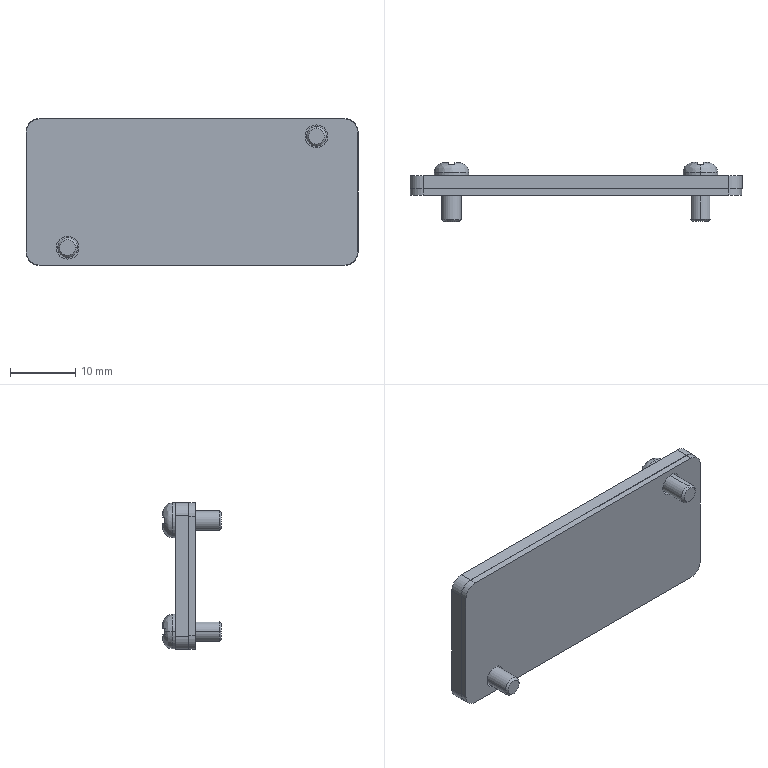Part | STEP file | P-200M-R2 AirTAC base blind plate assembly | 1 solid | 79 faces | box 50.7 x 9 x 22.4 mm | volume 3480 mm3 | plane 41 | cylinder 30 | spline 4 | cone 4 | commonest cylinder face diameters 4 x18 3 x4 3.5 x4 5.3 x4